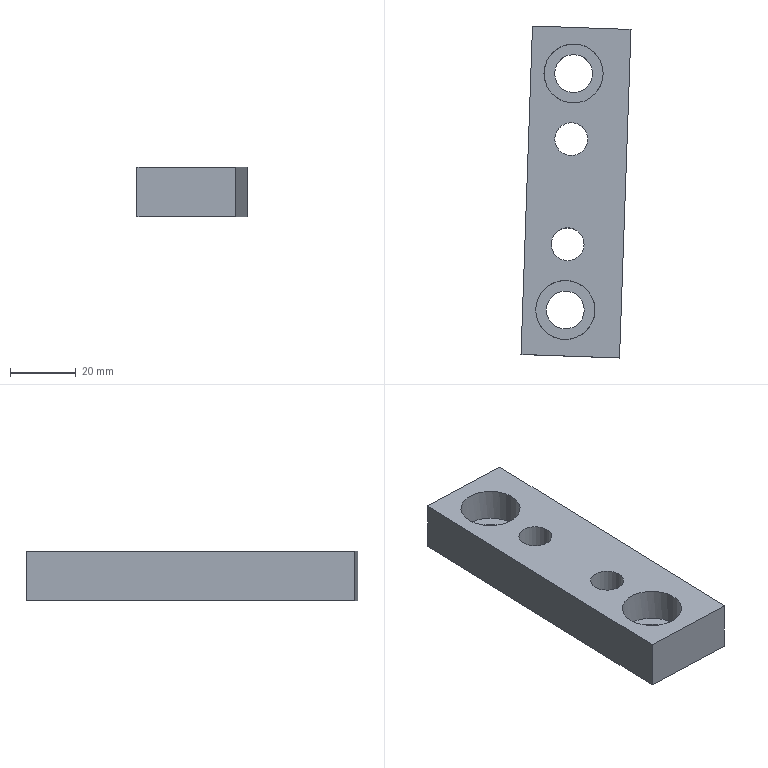Part | NX | features LB-11 2 | 1 solid | 14 faces | box 33.471 x 100.986 x 15 mm | volume 36516 mm3 | plane 8 | cylinder 6 | commonest cylinder face diameters 10 x2 11.5 x2 18 x2
STEP:
#1=CARTESIAN_POINT('',(3735.733,-918.048,818.716));
#2=VERTEX_POINT('',#1);
#3=CARTESIAN_POINT('',(3765.714,-919.095,818.716));
#4=VERTEX_POINT('',#3);
#5=CARTESIAN_POINT('',(3760.717,-918.92,818.716));
#6=DIRECTION('',(0.9994,-0.0349,0.000000002));
#7=VECTOR('',#6,1000.);
#8=LINE('',#5,#7);
#9=EDGE_CURVE('',#2,#4,#8,.T.);
#10=ORIENTED_EDGE('',*,*,#9,.F.);
#11=CARTESIAN_POINT('',(3735.733,-918.048,833.716));
#12=VERTEX_POINT('',#11);
#13=CARTESIAN_POINT('',(3735.733,-918.048,804.416));
#14=DIRECTION('',(0.000000002,0.,-1.));
#15=VECTOR('',#14,1000.);
#16=LINE('',#13,#15);
#17=EDGE_CURVE('',#2,#12,#16,.F.);
#18=ORIENTED_EDGE('',*,*,#17,.T.);
#19=CARTESIAN_POINT('',(3765.714,-919.095,833.716));
#20=VERTEX_POINT('',#19);
#21=CARTESIAN_POINT('',(3760.717,-918.92,833.716));
#22=DIRECTION('',(0.9994,-0.0349,0.000000002));
#23=VECTOR('',#22,1000.);
#24=LINE('',#21,#23);
#25=EDGE_CURVE('',#12,#20,#24,.T.);
#26=ORIENTED_EDGE('',*,*,#25,.T.);
#27=CARTESIAN_POINT('',(3765.714,-919.095,819.416));
#28=DIRECTION('',(0.000000002,0.,-1.));
#29=VECTOR('',#28,1000.);
#30=LINE('',#27,#29);
#31=EDGE_CURVE('',#20,#4,#30,.T.);
#32=ORIENTED_EDGE('',*,*,#31,.T.);
#33=EDGE_LOOP('',(#10,#18,#26,#32));
#34=FACE_BOUND('',#33,.T.);
#35=CARTESIAN_POINT('',(3760.717,-918.92,804.416));
#36=DIRECTION('',(0.0349,0.9994,0.));
#37=DIRECTION('',(-0.000000002,0.,1.));
#38=AXIS2_PLACEMENT_3D('',#35,#36,#37);
#39=PLANE('',#38);
#40=ADVANCED_FACE('',(#34),#39,.T.);
#41=CARTESIAN_POINT('',(3732.243,-1017.987,833.716));
#42=VERTEX_POINT('',#41);
#43=CARTESIAN_POINT('',(3732.243,-1017.987,818.716));
#44=VERTEX_POINT('',#43);
#45=CARTESIAN_POINT('',(3732.243,-1017.987,841.096));
#46=DIRECTION('',(-0.000000002,0.,1.));
#47=VECTOR('',#46,1000.);
#48=LINE('',#45,#47);
#49=EDGE_CURVE('',#42,#44,#48,.F.);
#50=ORIENTED_EDGE('',*,*,#49,.T.);
#51=CARTESIAN_POINT('',(3762.225,-1019.034,818.716));
#52=VERTEX_POINT('',#51);
#53=CARTESIAN_POINT('',(3717.083,-1017.458,818.716));
#54=DIRECTION('',(0.9994,-0.0349,0.000000002));
#55=VECTOR('',#54,1000.);
#56=LINE('',#53,#55);
#57=EDGE_CURVE('',#44,#52,#56,.T.);
#58=ORIENTED_EDGE('',*,*,#57,.T.);
#59=CARTESIAN_POINT('',(3762.225,-1019.034,833.716));
#60=VERTEX_POINT('',#59);
#61=CARTESIAN_POINT('',(3762.225,-1019.034,819.416));
#62=DIRECTION('',(-0.000000002,0.,1.));
#63=VECTOR('',#62,1000.);
#64=LINE('',#61,#63);
#65=EDGE_CURVE('',#60,#52,#64,.F.);
#66=ORIENTED_EDGE('',*,*,#65,.F.);
#67=CARTESIAN_POINT('',(3717.083,-1017.458,833.716));
#68=DIRECTION('',(0.9994,-0.0349,0.000000002));
#69=VECTOR('',#68,1000.);
#70=LINE('',#67,#69);
#71=EDGE_CURVE('',#42,#60,#70,.T.);
#72=ORIENTED_EDGE('',*,*,#71,.F.);
#73=EDGE_LOOP('',(#50,#58,#66,#72));
#74=FACE_BOUND('',#73,.T.);
#75=CARTESIAN_POINT('',(3757.228,-1018.86,841.096));
#76=DIRECTION('',(-0.0349,-0.9994,0.));
#77=DIRECTION('',(0.000000002,0.,-1.));
#78=AXIS2_PLACEMENT_3D('',#75,#76,#77);
#79=PLANE('',#78);
#80=ADVANCED_FACE('',(#74),#79,.T.);
#81=ORIENTED_EDGE('',*,*,#17,.F.);
#82=CARTESIAN_POINT('',(3734.965,-940.035,818.716));
#83=DIRECTION('',(-0.0349,-0.9994,0.));
#84=VECTOR('',#83,1000.);
#85=LINE('',#82,#84);
#86=EDGE_CURVE('',#2,#44,#85,.T.);
#87=ORIENTED_EDGE('',*,*,#86,.T.);
#88=ORIENTED_EDGE('',*,*,#49,.F.);
#89=CARTESIAN_POINT('',(3742.721,-717.906,833.716));
#90=DIRECTION('',(-0.0349,-0.9994,0.));
#91=VECTOR('',#90,1000.);
#92=LINE('',#89,#91);
#93=EDGE_CURVE('',#42,#12,#92,.F.);
#94=ORIENTED_EDGE('',*,*,#93,.T.);
#95=EDGE_LOOP('',(#81,#87,#88,#94));
#96=FACE_BOUND('',#95,.T.);
#97=CARTESIAN_POINT('',(3734.965,-940.035,821.416));
#98=DIRECTION('',(-0.9994,0.0349,-0.000000002));
#99=DIRECTION('',(0.0349,0.9994,0.));
#100=AXIS2_PLACEMENT_3D('',#97,#98,#99);
#101=PLANE('',#100);
#102=ADVANCED_FACE('',(#96),#101,.T.);
#103=CARTESIAN_POINT('',(3752.538,-952.481,818.716));
#104=VERTEX_POINT('',#103);
#105=CARTESIAN_POINT('',(3747.538,-952.481,818.716));
#106=DIRECTION('',(-0.000000002,0.,1.));
#107=DIRECTION('',(1.,0.,0.000000002));
#108=AXIS2_PLACEMENT_3D('',#105,#106,#107);
#109=CIRCLE('',#108,5.);
#110=EDGE_CURVE('',#104,#104,#109,.F.);
#111=ORIENTED_EDGE('',*,*,#110,.F.);
#112=EDGE_LOOP('',(#111));
#113=FACE_BOUND('',#112,.T.);
#114=CARTESIAN_POINT('',(3751.422,-984.461,818.716));
#115=VERTEX_POINT('',#114);
#116=CARTESIAN_POINT('',(3746.421,-984.461,818.716));
#117=DIRECTION('',(-0.000000002,0.,1.));
#118=DIRECTION('',(1.,0.,0.000000002));
#119=AXIS2_PLACEMENT_3D('',#116,#117,#118);
#120=CIRCLE('',#119,5.);
#121=EDGE_CURVE('',#115,#115,#120,.F.);
#122=ORIENTED_EDGE('',*,*,#121,.F.);
#123=EDGE_LOOP('',(#122));
#124=FACE_BOUND('',#123,.T.);
#125=CARTESIAN_POINT('',(3753.986,-932.493,818.716));
#126=VERTEX_POINT('',#125);
#127=CARTESIAN_POINT('',(3748.236,-932.493,818.716));
#128=DIRECTION('',(-0.000000002,0.,1.));
#129=DIRECTION('',(1.,0.,0.000000002));
#130=AXIS2_PLACEMENT_3D('',#127,#128,#129);
#131=CIRCLE('',#130,5.75);
#132=EDGE_CURVE('',#126,#126,#131,.F.);
#133=ORIENTED_EDGE('',*,*,#132,.F.);
#134=EDGE_LOOP('',(#133));
#135=FACE_BOUND('',#134,.T.);
#136=CARTESIAN_POINT('',(3751.474,-1004.449,818.716));
#137=VERTEX_POINT('',#136);
#138=CARTESIAN_POINT('',(3745.724,-1004.449,818.716));
#139=DIRECTION('',(-0.000000002,0.,1.));
#140=DIRECTION('',(1.,0.,0.000000002));
#141=AXIS2_PLACEMENT_3D('',#138,#139,#140);
#142=CIRCLE('',#141,5.75);
#143=EDGE_CURVE('',#137,#137,#142,.F.);
#144=ORIENTED_EDGE('',*,*,#143,.F.);
#145=EDGE_LOOP('',(#144));
#146=FACE_BOUND('',#145,.T.);
#147=ORIENTED_EDGE('',*,*,#57,.F.);
#148=ORIENTED_EDGE('',*,*,#86,.F.);
#149=ORIENTED_EDGE('',*,*,#9,.T.);
#150=CARTESIAN_POINT('',(3772.703,-718.953,818.716));
#151=DIRECTION('',(0.0349,0.9994,0.));
#152=VECTOR('',#151,1000.);
#153=LINE('',#150,#152);
#154=EDGE_CURVE('',#52,#4,#153,.T.);
#155=ORIENTED_EDGE('',*,*,#154,.F.);
#156=EDGE_LOOP('',(#147,#148,#149,#155));
#157=FACE_BOUND('',#156,.T.);
#158=CARTESIAN_POINT('',(3727.561,-717.377,818.716));
#159=DIRECTION('',(-0.000000002,0.,1.));
#160=DIRECTION('',(-0.8173,0.5762,-0.000000002));
#161=AXIS2_PLACEMENT_3D('',#158,#159,#160);
#162=PLANE('',#161);
#163=ADVANCED_FACE('',(#113,#124,#135,#146,#157),#162,.F.);
#164=CARTESIAN_POINT('',(3772.703,-718.953,833.716));
#165=DIRECTION('',(0.0349,0.9994,0.));
#166=VECTOR('',#165,1000.);
#167=LINE('',#164,#166);
#168=EDGE_CURVE('',#60,#20,#167,.T.);
#169=ORIENTED_EDGE('',*,*,#168,.F.);
#170=ORIENTED_EDGE('',*,*,#65,.T.);
#171=ORIENTED_EDGE('',*,*,#154,.T.);
#172=ORIENTED_EDGE('',*,*,#31,.F.);
#173=EDGE_LOOP('',(#169,#170,#171,#172));
#174=FACE_BOUND('',#173,.T.);
#175=CARTESIAN_POINT('',(3764.947,-941.082,819.416));
#176=DIRECTION('',(0.9994,-0.0349,0.000000002));
#177=DIRECTION('',(-0.0349,-0.9994,0.));
#178=AXIS2_PLACEMENT_3D('',#175,#176,#177);
#179=PLANE('',#178);
#180=ADVANCED_FACE('',(#174),#179,.T.);
#181=CARTESIAN_POINT('',(3752.538,-952.481,833.716));
#182=VERTEX_POINT('',#181);
#183=CARTESIAN_POINT('',(3747.538,-952.481,833.716));
#184=DIRECTION('',(-0.000000002,0.,1.));
#185=DIRECTION('',(1.,0.,0.000000002));
#186=AXIS2_PLACEMENT_3D('',#183,#184,#185);
#187=CIRCLE('',#186,5.);
#188=EDGE_CURVE('',#182,#182,#187,.F.);
#189=ORIENTED_EDGE('',*,*,#188,.T.);
#190=EDGE_LOOP('',(#189));
#191=FACE_BOUND('',#190,.T.);
#192=CARTESIAN_POINT('',(3751.422,-984.461,833.716));
#193=VERTEX_POINT('',#192);
#194=CARTESIAN_POINT('',(3746.421,-984.461,833.716));
#195=DIRECTION('',(-0.000000002,0.,1.));
#196=DIRECTION('',(1.,0.,0.000000002));
#197=AXIS2_PLACEMENT_3D('',#194,#195,#196);
#198=CIRCLE('',#197,5.);
#199=EDGE_CURVE('',#193,#193,#198,.F.);
#200=ORIENTED_EDGE('',*,*,#199,.T.);
#201=EDGE_LOOP('',(#200));
#202=FACE_BOUND('',#201,.T.);
#203=CARTESIAN_POINT('',(3757.236,-932.493,833.716));
#204=VERTEX_POINT('',#203);
#205=CARTESIAN_POINT('',(3748.236,-932.493,833.716));
#206=DIRECTION('',(-0.000000002,0.,1.));
#207=DIRECTION('',(1.,0.,0.000000002));
#208=AXIS2_PLACEMENT_3D('',#205,#206,#207);
#209=CIRCLE('',#208,9.);
#210=EDGE_CURVE('',#204,#204,#209,.F.);
#211=ORIENTED_EDGE('',*,*,#210,.T.);
#212=EDGE_LOOP('',(#211));
#213=FACE_BOUND('',#212,.T.);
#214=CARTESIAN_POINT('',(3754.724,-1004.449,833.716));
#215=VERTEX_POINT('',#214);
#216=CARTESIAN_POINT('',(3745.724,-1004.449,833.716));
#217=DIRECTION('',(-0.000000002,0.,1.));
#218=DIRECTION('',(1.,0.,0.000000002));
#219=AXIS2_PLACEMENT_3D('',#216,#217,#218);
#220=CIRCLE('',#219,9.);
#221=EDGE_CURVE('',#215,#215,#220,.F.);
#222=ORIENTED_EDGE('',*,*,#221,.T.);
#223=EDGE_LOOP('',(#222));
#224=FACE_BOUND('',#223,.T.);
#225=ORIENTED_EDGE('',*,*,#25,.F.);
#226=ORIENTED_EDGE('',*,*,#93,.F.);
#227=ORIENTED_EDGE('',*,*,#71,.T.);
#228=ORIENTED_EDGE('',*,*,#168,.T.);
#229=EDGE_LOOP('',(#225,#226,#227,#228));
#230=FACE_BOUND('',#229,.T.);
#231=CARTESIAN_POINT('',(3727.561,-717.377,833.716));
#232=DIRECTION('',(-0.000000002,0.,1.));
#233=DIRECTION('',(-0.8173,0.5762,-0.000000002));
#234=AXIS2_PLACEMENT_3D('',#231,#232,#233);
#235=PLANE('',#234);
#236=ADVANCED_FACE('',(#191,#202,#213,#224,#230),#235,.T.);
#237=CARTESIAN_POINT('',(3746.038,-995.455,823.716));
#238=VERTEX_POINT('',#237);
#239=CARTESIAN_POINT('',(3745.724,-1004.449,823.716));
#240=DIRECTION('',(-0.000000002,0.,1.));
#241=DIRECTION('',(0.0349,0.9994,0.));
#242=AXIS2_PLACEMENT_3D('',#239,#240,#241);
#243=CIRCLE('',#242,9.);
#244=EDGE_CURVE('',#238,#238,#243,.F.);
#245=ORIENTED_EDGE('',*,*,#244,.T.);
#246=EDGE_LOOP('',(#245));
#247=FACE_BOUND('',#246,.T.);
#248=ORIENTED_EDGE('',*,*,#221,.F.);
#249=EDGE_LOOP('',(#248));
#250=FACE_BOUND('',#249,.T.);
#251=CARTESIAN_POINT('',(3745.724,-1004.449,823.716));
#252=DIRECTION('',(-0.000000002,0.,1.));
#253=DIRECTION('',(1.,0.,0.000000002));
#254=AXIS2_PLACEMENT_3D('',#251,#252,#253);
#255=CYLINDRICAL_SURFACE('',#254,9.);
#256=ADVANCED_FACE('',(#247,#250),#255,.F.);
#257=ORIENTED_EDGE('',*,*,#143,.T.);
#258=EDGE_LOOP('',(#257));
#259=FACE_BOUND('',#258,.T.);
#260=CARTESIAN_POINT('',(3751.474,-1004.449,823.716));
#261=VERTEX_POINT('',#260);
#262=CARTESIAN_POINT('',(3745.724,-1004.449,823.716));
#263=DIRECTION('',(-0.000000002,0.,1.));
#264=DIRECTION('',(1.,0.,0.000000002));
#265=AXIS2_PLACEMENT_3D('',#262,#263,#264);
#266=CIRCLE('',#265,5.75);
#267=EDGE_CURVE('',#261,#261,#266,.T.);
#268=ORIENTED_EDGE('',*,*,#267,.T.);
#269=EDGE_LOOP('',(#268));
#270=FACE_BOUND('',#269,.T.);
#271=CARTESIAN_POINT('',(3745.724,-1004.449,817.716));
#272=DIRECTION('',(-0.000000002,0.,1.));
#273=DIRECTION('',(1.,0.,0.000000002));
#274=AXIS2_PLACEMENT_3D('',#271,#272,#273);
#275=CYLINDRICAL_SURFACE('',#274,5.75);
#276=ADVANCED_FACE('',(#259,#270),#275,.F.);
#277=ORIENTED_EDGE('',*,*,#267,.F.);
#278=EDGE_LOOP('',(#277));
#279=FACE_BOUND('',#278,.T.);
#280=ORIENTED_EDGE('',*,*,#244,.F.);
#281=EDGE_LOOP('',(#280));
#282=FACE_BOUND('',#281,.T.);
#283=CARTESIAN_POINT('',(3745.724,-1004.449,823.716));
#284=DIRECTION('',(-0.000000002,0.,1.));
#285=DIRECTION('',(1.,0.,0.000000002));
#286=AXIS2_PLACEMENT_3D('',#283,#284,#285);
#287=PLANE('',#286);
#288=ADVANCED_FACE('',(#279,#282),#287,.T.);
#289=CARTESIAN_POINT('',(3748.55,-923.499,823.716));
#290=VERTEX_POINT('',#289);
#291=CARTESIAN_POINT('',(3748.236,-932.493,823.716));
#292=DIRECTION('',(-0.000000002,0.,1.));
#293=DIRECTION('',(0.0349,0.9994,0.));
#294=AXIS2_PLACEMENT_3D('',#291,#292,#293);
#295=CIRCLE('',#294,9.);
#296=EDGE_CURVE('',#290,#290,#295,.F.);
#297=ORIENTED_EDGE('',*,*,#296,.T.);
#298=EDGE_LOOP('',(#297));
#299=FACE_BOUND('',#298,.T.);
#300=ORIENTED_EDGE('',*,*,#210,.F.);
#301=EDGE_LOOP('',(#300));
#302=FACE_BOUND('',#301,.T.);
#303=CARTESIAN_POINT('',(3748.236,-932.493,823.716));
#304=DIRECTION('',(-0.000000002,0.,1.));
#305=DIRECTION('',(1.,0.,0.000000002));
#306=AXIS2_PLACEMENT_3D('',#303,#304,#305);
#307=CYLINDRICAL_SURFACE('',#306,9.);
#308=ADVANCED_FACE('',(#299,#302),#307,.F.);
#309=ORIENTED_EDGE('',*,*,#132,.T.);
#310=EDGE_LOOP('',(#309));
#311=FACE_BOUND('',#310,.T.);
#312=CARTESIAN_POINT('',(3753.986,-932.493,823.716));
#313=VERTEX_POINT('',#312);
#314=CARTESIAN_POINT('',(3748.236,-932.493,823.716));
#315=DIRECTION('',(-0.000000002,0.,1.));
#316=DIRECTION('',(1.,0.,0.000000002));
#317=AXIS2_PLACEMENT_3D('',#314,#315,#316);
#318=CIRCLE('',#317,5.75);
#319=EDGE_CURVE('',#313,#313,#318,.T.);
#320=ORIENTED_EDGE('',*,*,#319,.T.);
#321=EDGE_LOOP('',(#320));
#322=FACE_BOUND('',#321,.T.);
#323=CARTESIAN_POINT('',(3748.236,-932.493,817.716));
#324=DIRECTION('',(-0.000000002,0.,1.));
#325=DIRECTION('',(1.,0.,0.000000002));
#326=AXIS2_PLACEMENT_3D('',#323,#324,#325);
#327=CYLINDRICAL_SURFACE('',#326,5.75);
#328=ADVANCED_FACE('',(#311,#322),#327,.F.);
#329=ORIENTED_EDGE('',*,*,#319,.F.);
#330=EDGE_LOOP('',(#329));
#331=FACE_BOUND('',#330,.T.);
#332=ORIENTED_EDGE('',*,*,#296,.F.);
#333=EDGE_LOOP('',(#332));
#334=FACE_BOUND('',#333,.T.);
#335=CARTESIAN_POINT('',(3748.236,-932.493,823.716));
#336=DIRECTION('',(-0.000000002,0.,1.));
#337=DIRECTION('',(1.,0.,0.000000002));
#338=AXIS2_PLACEMENT_3D('',#335,#336,#337);
#339=PLANE('',#338);
#340=ADVANCED_FACE('',(#331,#334),#339,.T.);
#341=ORIENTED_EDGE('',*,*,#121,.T.);
#342=EDGE_LOOP('',(#341));
#343=FACE_BOUND('',#342,.T.);
#344=ORIENTED_EDGE('',*,*,#199,.F.);
#345=EDGE_LOOP('',(#344));
#346=FACE_BOUND('',#345,.T.);
#347=CARTESIAN_POINT('',(3746.421,-984.461,817.716));
#348=DIRECTION('',(-0.000000002,0.,1.));
#349=DIRECTION('',(1.,0.,0.000000002));
#350=AXIS2_PLACEMENT_3D('',#347,#348,#349);
#351=CYLINDRICAL_SURFACE('',#350,5.);
#352=ADVANCED_FACE('',(#343,#346),#351,.F.);
#353=ORIENTED_EDGE('',*,*,#110,.T.);
#354=EDGE_LOOP('',(#353));
#355=FACE_BOUND('',#354,.T.);
#356=ORIENTED_EDGE('',*,*,#188,.F.);
#357=EDGE_LOOP('',(#356));
#358=FACE_BOUND('',#357,.T.);
#359=CARTESIAN_POINT('',(3747.538,-952.481,817.716));
#360=DIRECTION('',(-0.000000002,0.,1.));
#361=DIRECTION('',(1.,0.,0.000000002));
#362=AXIS2_PLACEMENT_3D('',#359,#360,#361);
#363=CYLINDRICAL_SURFACE('',#362,5.);
#364=ADVANCED_FACE('',(#355,#358),#363,.F.);
#365=CLOSED_SHELL('',(#40,#80,#102,#163,#180,#236,#256,#276,#288,#308,#328,#340,#352,#364));
#366=MANIFOLD_SOLID_BREP('',#365);
#367=(LENGTH_UNIT()NAMED_UNIT(*)SI_UNIT(.MILLI.,.METRE.));
#368=UNCERTAINTY_MEASURE_WITH_UNIT(LENGTH_MEASURE(0.00001),#367,'','');
#369=(NAMED_UNIT(*)PLANE_ANGLE_UNIT()SI_UNIT($,.RADIAN.));
#370=(NAMED_UNIT(*)SI_UNIT($,.STERADIAN.)SOLID_ANGLE_UNIT());
#371=(GEOMETRIC_REPRESENTATION_CONTEXT(3)GLOBAL_UNCERTAINTY_ASSIGNED_CONTEXT((#368))GLOBAL_UNIT_ASSIGNED_CONTEXT((#367,#369,#370))REPRESENTATION_CONTEXT('',''));
#372=ADVANCED_BREP_SHAPE_REPRESENTATION('',(#366),#371);